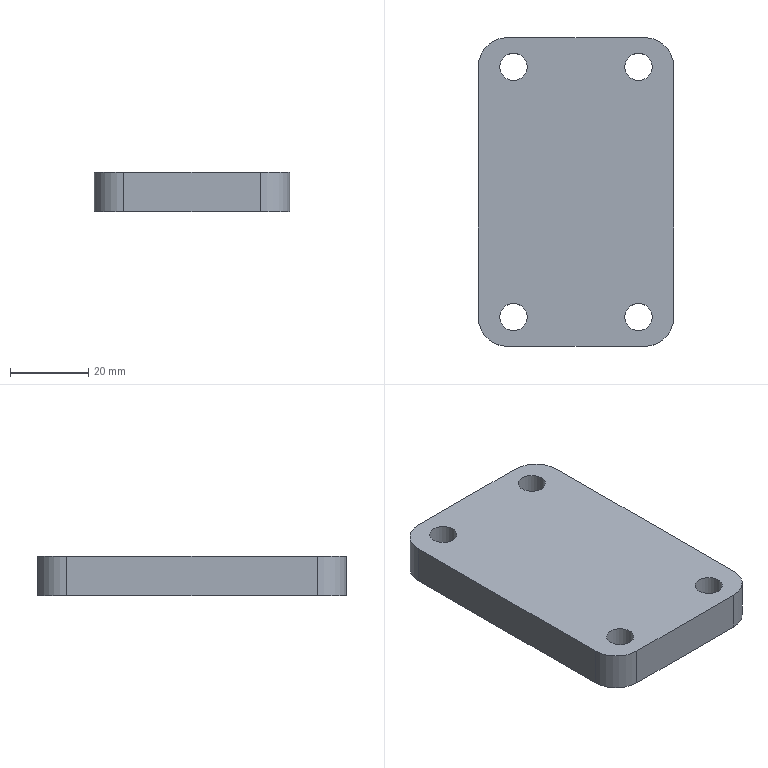Part | NX | features solid 2 | 1 solid | 14 faces | box 50 x 79 x 10 mm | volume 37478 mm3 | cylinder 8 | plane 6 | commonest cylinder face diameters 7 x4 15 x4
STEP:
#1=CARTESIAN_POINT('',(-542.5,-19.5,-137.));
#2=VERTEX_POINT('',#1);
#3=CARTESIAN_POINT('',(-577.5,-19.5,-137.));
#4=VERTEX_POINT('',#3);
#5=CARTESIAN_POINT('',(-535.,-19.5,-137.));
#6=DIRECTION('',(-1.,0.,0.));
#7=VECTOR('',#6,1000.);
#8=LINE('',#5,#7);
#9=EDGE_CURVE('',#2,#4,#8,.T.);
#10=ORIENTED_EDGE('',*,*,#9,.T.);
#11=CARTESIAN_POINT('',(-577.5,-19.5,-147.));
#12=VERTEX_POINT('',#11);
#13=CARTESIAN_POINT('',(-577.5,-19.5,-137.));
#14=DIRECTION('',(0.,0.,-1.));
#15=VECTOR('',#14,1000.);
#16=LINE('',#13,#15);
#17=EDGE_CURVE('',#4,#12,#16,.T.);
#18=ORIENTED_EDGE('',*,*,#17,.T.);
#19=CARTESIAN_POINT('',(-542.5,-19.5,-147.));
#20=VERTEX_POINT('',#19);
#21=CARTESIAN_POINT('',(-535.,-19.5,-147.));
#22=DIRECTION('',(-1.,0.,0.));
#23=VECTOR('',#22,1000.);
#24=LINE('',#21,#23);
#25=EDGE_CURVE('',#20,#12,#24,.T.);
#26=ORIENTED_EDGE('',*,*,#25,.F.);
#27=CARTESIAN_POINT('',(-542.5,-19.5,-137.));
#28=DIRECTION('',(0.,0.,-1.));
#29=VECTOR('',#28,1000.);
#30=LINE('',#27,#29);
#31=EDGE_CURVE('',#20,#2,#30,.F.);
#32=ORIENTED_EDGE('',*,*,#31,.T.);
#33=EDGE_LOOP('',(#10,#18,#26,#32));
#34=FACE_BOUND('',#33,.T.);
#35=CARTESIAN_POINT('',(-535.,-19.5,-137.));
#36=DIRECTION('',(0.,-1.,0.));
#37=DIRECTION('',(1.,0.,0.));
#38=AXIS2_PLACEMENT_3D('',#35,#36,#37);
#39=PLANE('',#38);
#40=ADVANCED_FACE('',(#34),#39,.T.);
#41=CARTESIAN_POINT('',(-585.,-12.,-137.));
#42=VERTEX_POINT('',#41);
#43=CARTESIAN_POINT('',(-585.,52.,-137.));
#44=VERTEX_POINT('',#43);
#45=CARTESIAN_POINT('',(-585.,-19.5,-137.));
#46=DIRECTION('',(0.,1.,0.));
#47=VECTOR('',#46,1000.);
#48=LINE('',#45,#47);
#49=EDGE_CURVE('',#42,#44,#48,.T.);
#50=ORIENTED_EDGE('',*,*,#49,.T.);
#51=CARTESIAN_POINT('',(-585.,52.,-147.));
#52=VERTEX_POINT('',#51);
#53=CARTESIAN_POINT('',(-585.,52.,-137.));
#54=DIRECTION('',(0.,0.,-1.));
#55=VECTOR('',#54,1000.);
#56=LINE('',#53,#55);
#57=EDGE_CURVE('',#44,#52,#56,.T.);
#58=ORIENTED_EDGE('',*,*,#57,.T.);
#59=CARTESIAN_POINT('',(-585.,-12.,-147.));
#60=VERTEX_POINT('',#59);
#61=CARTESIAN_POINT('',(-585.,-19.5,-147.));
#62=DIRECTION('',(0.,1.,0.));
#63=VECTOR('',#62,1000.);
#64=LINE('',#61,#63);
#65=EDGE_CURVE('',#60,#52,#64,.T.);
#66=ORIENTED_EDGE('',*,*,#65,.F.);
#67=CARTESIAN_POINT('',(-585.,-12.,-137.));
#68=DIRECTION('',(0.,0.,-1.));
#69=VECTOR('',#68,1000.);
#70=LINE('',#67,#69);
#71=EDGE_CURVE('',#60,#42,#70,.F.);
#72=ORIENTED_EDGE('',*,*,#71,.T.);
#73=EDGE_LOOP('',(#50,#58,#66,#72));
#74=FACE_BOUND('',#73,.T.);
#75=CARTESIAN_POINT('',(-585.,-19.5,-137.));
#76=DIRECTION('',(-1.,0.,0.));
#77=DIRECTION('',(0.,-1.,0.));
#78=AXIS2_PLACEMENT_3D('',#75,#76,#77);
#79=PLANE('',#78);
#80=ADVANCED_FACE('',(#74),#79,.T.);
#81=CARTESIAN_POINT('',(-577.5,59.5,-147.));
#82=VERTEX_POINT('',#81);
#83=CARTESIAN_POINT('',(-542.5,59.5,-147.));
#84=VERTEX_POINT('',#83);
#85=CARTESIAN_POINT('',(-585.,59.5,-147.));
#86=DIRECTION('',(1.,0.,0.));
#87=VECTOR('',#86,1000.);
#88=LINE('',#85,#87);
#89=EDGE_CURVE('',#82,#84,#88,.T.);
#90=ORIENTED_EDGE('',*,*,#89,.F.);
#91=CARTESIAN_POINT('',(-577.5,59.5,-137.));
#92=VERTEX_POINT('',#91);
#93=CARTESIAN_POINT('',(-577.5,59.5,-137.));
#94=DIRECTION('',(0.,0.,-1.));
#95=VECTOR('',#94,1000.);
#96=LINE('',#93,#95);
#97=EDGE_CURVE('',#82,#92,#96,.F.);
#98=ORIENTED_EDGE('',*,*,#97,.T.);
#99=CARTESIAN_POINT('',(-542.5,59.5,-137.));
#100=VERTEX_POINT('',#99);
#101=CARTESIAN_POINT('',(-585.,59.5,-137.));
#102=DIRECTION('',(1.,0.,0.));
#103=VECTOR('',#102,1000.);
#104=LINE('',#101,#103);
#105=EDGE_CURVE('',#92,#100,#104,.T.);
#106=ORIENTED_EDGE('',*,*,#105,.T.);
#107=CARTESIAN_POINT('',(-542.5,59.5,-137.));
#108=DIRECTION('',(0.,0.,-1.));
#109=VECTOR('',#108,1000.);
#110=LINE('',#107,#109);
#111=EDGE_CURVE('',#100,#84,#110,.T.);
#112=ORIENTED_EDGE('',*,*,#111,.T.);
#113=EDGE_LOOP('',(#90,#98,#106,#112));
#114=FACE_BOUND('',#113,.T.);
#115=CARTESIAN_POINT('',(-585.,59.5,-137.));
#116=DIRECTION('',(0.,1.,0.));
#117=DIRECTION('',(-1.,0.,0.));
#118=AXIS2_PLACEMENT_3D('',#115,#116,#117);
#119=PLANE('',#118);
#120=ADVANCED_FACE('',(#114),#119,.T.);
#121=CARTESIAN_POINT('',(-535.,52.,-147.));
#122=VERTEX_POINT('',#121);
#123=CARTESIAN_POINT('',(-535.,-12.,-147.));
#124=VERTEX_POINT('',#123);
#125=CARTESIAN_POINT('',(-535.,59.5,-147.));
#126=DIRECTION('',(0.,-1.,0.));
#127=VECTOR('',#126,1000.);
#128=LINE('',#125,#127);
#129=EDGE_CURVE('',#122,#124,#128,.T.);
#130=ORIENTED_EDGE('',*,*,#129,.F.);
#131=CARTESIAN_POINT('',(-535.,52.,-137.));
#132=VERTEX_POINT('',#131);
#133=CARTESIAN_POINT('',(-535.,52.,-137.));
#134=DIRECTION('',(0.,0.,-1.));
#135=VECTOR('',#134,1000.);
#136=LINE('',#133,#135);
#137=EDGE_CURVE('',#122,#132,#136,.F.);
#138=ORIENTED_EDGE('',*,*,#137,.T.);
#139=CARTESIAN_POINT('',(-535.,-12.,-137.));
#140=VERTEX_POINT('',#139);
#141=CARTESIAN_POINT('',(-535.,59.5,-137.));
#142=DIRECTION('',(0.,-1.,0.));
#143=VECTOR('',#142,1000.);
#144=LINE('',#141,#143);
#145=EDGE_CURVE('',#132,#140,#144,.T.);
#146=ORIENTED_EDGE('',*,*,#145,.T.);
#147=CARTESIAN_POINT('',(-535.,-12.,-137.));
#148=DIRECTION('',(0.,0.,-1.));
#149=VECTOR('',#148,1000.);
#150=LINE('',#147,#149);
#151=EDGE_CURVE('',#140,#124,#150,.T.);
#152=ORIENTED_EDGE('',*,*,#151,.T.);
#153=EDGE_LOOP('',(#130,#138,#146,#152));
#154=FACE_BOUND('',#153,.T.);
#155=CARTESIAN_POINT('',(-535.,59.5,-137.));
#156=DIRECTION('',(1.,0.,0.));
#157=DIRECTION('',(0.,1.,0.));
#158=AXIS2_PLACEMENT_3D('',#155,#156,#157);
#159=PLANE('',#158);
#160=ADVANCED_FACE('',(#154),#159,.T.);
#161=CARTESIAN_POINT('',(-544.,55.5,-137.));
#162=VERTEX_POINT('',#161);
#163=CARTESIAN_POINT('',(-544.,52.,-137.));
#164=DIRECTION('',(0.,0.,-1.));
#165=DIRECTION('',(0.,1.,0.));
#166=AXIS2_PLACEMENT_3D('',#163,#164,#165);
#167=CIRCLE('',#166,3.5);
#168=EDGE_CURVE('',#162,#162,#167,.T.);
#169=ORIENTED_EDGE('',*,*,#168,.T.);
#170=EDGE_LOOP('',(#169));
#171=FACE_BOUND('',#170,.T.);
#172=CARTESIAN_POINT('',(-576.,55.5,-137.));
#173=VERTEX_POINT('',#172);
#174=CARTESIAN_POINT('',(-576.,52.,-137.));
#175=DIRECTION('',(0.,0.,1.));
#176=DIRECTION('',(0.,1.,0.));
#177=AXIS2_PLACEMENT_3D('',#174,#175,#176);
#178=CIRCLE('',#177,3.5);
#179=EDGE_CURVE('',#173,#173,#178,.T.);
#180=ORIENTED_EDGE('',*,*,#179,.F.);
#181=EDGE_LOOP('',(#180));
#182=FACE_BOUND('',#181,.T.);
#183=CARTESIAN_POINT('',(-544.,-15.5,-137.));
#184=VERTEX_POINT('',#183);
#185=CARTESIAN_POINT('',(-544.,-12.,-137.));
#186=DIRECTION('',(0.,0.,1.));
#187=DIRECTION('',(0.,-1.,0.));
#188=AXIS2_PLACEMENT_3D('',#185,#186,#187);
#189=CIRCLE('',#188,3.5);
#190=EDGE_CURVE('',#184,#184,#189,.T.);
#191=ORIENTED_EDGE('',*,*,#190,.F.);
#192=EDGE_LOOP('',(#191));
#193=FACE_BOUND('',#192,.T.);
#194=CARTESIAN_POINT('',(-576.,-15.5,-137.));
#195=VERTEX_POINT('',#194);
#196=CARTESIAN_POINT('',(-576.,-12.,-137.));
#197=DIRECTION('',(0.,0.,-1.));
#198=DIRECTION('',(0.,-1.,0.));
#199=AXIS2_PLACEMENT_3D('',#196,#197,#198);
#200=CIRCLE('',#199,3.5);
#201=EDGE_CURVE('',#195,#195,#200,.T.);
#202=ORIENTED_EDGE('',*,*,#201,.T.);
#203=EDGE_LOOP('',(#202));
#204=FACE_BOUND('',#203,.T.);
#205=ORIENTED_EDGE('',*,*,#105,.F.);
#206=CARTESIAN_POINT('',(-577.5,52.,-137.));
#207=DIRECTION('',(0.,0.,1.));
#208=DIRECTION('',(0.,1.,0.));
#209=AXIS2_PLACEMENT_3D('',#206,#207,#208);
#210=CIRCLE('',#209,7.5);
#211=EDGE_CURVE('',#92,#44,#210,.T.);
#212=ORIENTED_EDGE('',*,*,#211,.T.);
#213=ORIENTED_EDGE('',*,*,#49,.F.);
#214=CARTESIAN_POINT('',(-577.5,-12.,-137.));
#215=DIRECTION('',(0.,0.,1.));
#216=DIRECTION('',(0.,1.,0.));
#217=AXIS2_PLACEMENT_3D('',#214,#215,#216);
#218=CIRCLE('',#217,7.5);
#219=EDGE_CURVE('',#42,#4,#218,.T.);
#220=ORIENTED_EDGE('',*,*,#219,.T.);
#221=ORIENTED_EDGE('',*,*,#9,.F.);
#222=CARTESIAN_POINT('',(-542.5,-12.,-137.));
#223=DIRECTION('',(0.,0.,1.));
#224=DIRECTION('',(0.,1.,0.));
#225=AXIS2_PLACEMENT_3D('',#222,#223,#224);
#226=CIRCLE('',#225,7.5);
#227=EDGE_CURVE('',#2,#140,#226,.T.);
#228=ORIENTED_EDGE('',*,*,#227,.T.);
#229=ORIENTED_EDGE('',*,*,#145,.F.);
#230=CARTESIAN_POINT('',(-542.5,52.,-137.));
#231=DIRECTION('',(0.,0.,1.));
#232=DIRECTION('',(0.,1.,0.));
#233=AXIS2_PLACEMENT_3D('',#230,#231,#232);
#234=CIRCLE('',#233,7.5);
#235=EDGE_CURVE('',#132,#100,#234,.T.);
#236=ORIENTED_EDGE('',*,*,#235,.T.);
#237=EDGE_LOOP('',(#205,#212,#213,#220,#221,#228,#229,#236));
#238=FACE_BOUND('',#237,.T.);
#239=CARTESIAN_POINT('',(-535.,-19.5,-137.));
#240=DIRECTION('',(0.,0.,1.));
#241=DIRECTION('',(0.,1.,0.));
#242=AXIS2_PLACEMENT_3D('',#239,#240,#241);
#243=PLANE('',#242);
#244=ADVANCED_FACE('',(#171,#182,#193,#204,#238),#243,.T.);
#245=CARTESIAN_POINT('',(-544.,55.5,-147.));
#246=VERTEX_POINT('',#245);
#247=CARTESIAN_POINT('',(-544.,52.,-147.));
#248=DIRECTION('',(0.,0.,-1.));
#249=DIRECTION('',(0.,1.,0.));
#250=AXIS2_PLACEMENT_3D('',#247,#248,#249);
#251=CIRCLE('',#250,3.5);
#252=EDGE_CURVE('',#246,#246,#251,.T.);
#253=ORIENTED_EDGE('',*,*,#252,.F.);
#254=EDGE_LOOP('',(#253));
#255=FACE_BOUND('',#254,.T.);
#256=CARTESIAN_POINT('',(-576.,55.5,-147.));
#257=VERTEX_POINT('',#256);
#258=CARTESIAN_POINT('',(-576.,52.,-147.));
#259=DIRECTION('',(0.,0.,1.));
#260=DIRECTION('',(0.,1.,0.));
#261=AXIS2_PLACEMENT_3D('',#258,#259,#260);
#262=CIRCLE('',#261,3.5);
#263=EDGE_CURVE('',#257,#257,#262,.T.);
#264=ORIENTED_EDGE('',*,*,#263,.T.);
#265=EDGE_LOOP('',(#264));
#266=FACE_BOUND('',#265,.T.);
#267=CARTESIAN_POINT('',(-544.,-15.5,-147.));
#268=VERTEX_POINT('',#267);
#269=CARTESIAN_POINT('',(-544.,-12.,-147.));
#270=DIRECTION('',(0.,0.,1.));
#271=DIRECTION('',(0.,-1.,0.));
#272=AXIS2_PLACEMENT_3D('',#269,#270,#271);
#273=CIRCLE('',#272,3.5);
#274=EDGE_CURVE('',#268,#268,#273,.T.);
#275=ORIENTED_EDGE('',*,*,#274,.T.);
#276=EDGE_LOOP('',(#275));
#277=FACE_BOUND('',#276,.T.);
#278=CARTESIAN_POINT('',(-576.,-15.5,-147.));
#279=VERTEX_POINT('',#278);
#280=CARTESIAN_POINT('',(-576.,-12.,-147.));
#281=DIRECTION('',(0.,0.,-1.));
#282=DIRECTION('',(0.,-1.,0.));
#283=AXIS2_PLACEMENT_3D('',#280,#281,#282);
#284=CIRCLE('',#283,3.5);
#285=EDGE_CURVE('',#279,#279,#284,.T.);
#286=ORIENTED_EDGE('',*,*,#285,.F.);
#287=EDGE_LOOP('',(#286));
#288=FACE_BOUND('',#287,.T.);
#289=ORIENTED_EDGE('',*,*,#65,.T.);
#290=CARTESIAN_POINT('',(-577.5,52.,-147.));
#291=DIRECTION('',(0.,0.,1.));
#292=DIRECTION('',(0.,1.,0.));
#293=AXIS2_PLACEMENT_3D('',#290,#291,#292);
#294=CIRCLE('',#293,7.5);
#295=EDGE_CURVE('',#52,#82,#294,.F.);
#296=ORIENTED_EDGE('',*,*,#295,.T.);
#297=ORIENTED_EDGE('',*,*,#89,.T.);
#298=CARTESIAN_POINT('',(-542.5,52.,-147.));
#299=DIRECTION('',(0.,0.,1.));
#300=DIRECTION('',(0.,1.,0.));
#301=AXIS2_PLACEMENT_3D('',#298,#299,#300);
#302=CIRCLE('',#301,7.5);
#303=EDGE_CURVE('',#84,#122,#302,.F.);
#304=ORIENTED_EDGE('',*,*,#303,.T.);
#305=ORIENTED_EDGE('',*,*,#129,.T.);
#306=CARTESIAN_POINT('',(-542.5,-12.,-147.));
#307=DIRECTION('',(0.,0.,1.));
#308=DIRECTION('',(0.,1.,0.));
#309=AXIS2_PLACEMENT_3D('',#306,#307,#308);
#310=CIRCLE('',#309,7.5);
#311=EDGE_CURVE('',#124,#20,#310,.F.);
#312=ORIENTED_EDGE('',*,*,#311,.T.);
#313=ORIENTED_EDGE('',*,*,#25,.T.);
#314=CARTESIAN_POINT('',(-577.5,-12.,-147.));
#315=DIRECTION('',(0.,0.,1.));
#316=DIRECTION('',(0.,1.,0.));
#317=AXIS2_PLACEMENT_3D('',#314,#315,#316);
#318=CIRCLE('',#317,7.5);
#319=EDGE_CURVE('',#12,#60,#318,.F.);
#320=ORIENTED_EDGE('',*,*,#319,.T.);
#321=EDGE_LOOP('',(#289,#296,#297,#304,#305,#312,#313,#320));
#322=FACE_BOUND('',#321,.T.);
#323=CARTESIAN_POINT('',(-535.,-19.5,-147.));
#324=DIRECTION('',(0.,0.,1.));
#325=DIRECTION('',(0.,1.,0.));
#326=AXIS2_PLACEMENT_3D('',#323,#324,#325);
#327=PLANE('',#326);
#328=ADVANCED_FACE('',(#255,#266,#277,#288,#322),#327,.F.);
#329=ORIENTED_EDGE('',*,*,#211,.F.);
#330=ORIENTED_EDGE('',*,*,#97,.F.);
#331=ORIENTED_EDGE('',*,*,#295,.F.);
#332=ORIENTED_EDGE('',*,*,#57,.F.);
#333=EDGE_LOOP('',(#329,#330,#331,#332));
#334=FACE_BOUND('',#333,.T.);
#335=CARTESIAN_POINT('',(-577.5,52.,-137.));
#336=DIRECTION('',(0.,0.,-1.));
#337=DIRECTION('',(0.,-1.,0.));
#338=AXIS2_PLACEMENT_3D('',#335,#336,#337);
#339=CYLINDRICAL_SURFACE('',#338,7.5);
#340=ADVANCED_FACE('',(#334),#339,.T.);
#341=ORIENTED_EDGE('',*,*,#235,.F.);
#342=ORIENTED_EDGE('',*,*,#137,.F.);
#343=ORIENTED_EDGE('',*,*,#303,.F.);
#344=ORIENTED_EDGE('',*,*,#111,.F.);
#345=EDGE_LOOP('',(#341,#342,#343,#344));
#346=FACE_BOUND('',#345,.T.);
#347=CARTESIAN_POINT('',(-542.5,52.,-137.));
#348=DIRECTION('',(0.,0.,-1.));
#349=DIRECTION('',(0.,-1.,0.));
#350=AXIS2_PLACEMENT_3D('',#347,#348,#349);
#351=CYLINDRICAL_SURFACE('',#350,7.5);
#352=ADVANCED_FACE('',(#346),#351,.T.);
#353=ORIENTED_EDGE('',*,*,#219,.F.);
#354=ORIENTED_EDGE('',*,*,#71,.F.);
#355=ORIENTED_EDGE('',*,*,#319,.F.);
#356=ORIENTED_EDGE('',*,*,#17,.F.);
#357=EDGE_LOOP('',(#353,#354,#355,#356));
#358=FACE_BOUND('',#357,.T.);
#359=CARTESIAN_POINT('',(-577.5,-12.,-137.));
#360=DIRECTION('',(0.,0.,-1.));
#361=DIRECTION('',(0.,-1.,0.));
#362=AXIS2_PLACEMENT_3D('',#359,#360,#361);
#363=CYLINDRICAL_SURFACE('',#362,7.5);
#364=ADVANCED_FACE('',(#358),#363,.T.);
#365=ORIENTED_EDGE('',*,*,#227,.F.);
#366=ORIENTED_EDGE('',*,*,#31,.F.);
#367=ORIENTED_EDGE('',*,*,#311,.F.);
#368=ORIENTED_EDGE('',*,*,#151,.F.);
#369=EDGE_LOOP('',(#365,#366,#367,#368));
#370=FACE_BOUND('',#369,.T.);
#371=CARTESIAN_POINT('',(-542.5,-12.,-137.));
#372=DIRECTION('',(0.,0.,-1.));
#373=DIRECTION('',(0.,-1.,0.));
#374=AXIS2_PLACEMENT_3D('',#371,#372,#373);
#375=CYLINDRICAL_SURFACE('',#374,7.5);
#376=ADVANCED_FACE('',(#370),#375,.T.);
#377=ORIENTED_EDGE('',*,*,#285,.T.);
#378=EDGE_LOOP('',(#377));
#379=FACE_BOUND('',#378,.T.);
#380=ORIENTED_EDGE('',*,*,#201,.F.);
#381=EDGE_LOOP('',(#380));
#382=FACE_BOUND('',#381,.T.);
#383=CARTESIAN_POINT('',(-576.,-12.,-137.));
#384=DIRECTION('',(0.,0.,-1.));
#385=DIRECTION('',(0.,-1.,0.));
#386=AXIS2_PLACEMENT_3D('',#383,#384,#385);
#387=CYLINDRICAL_SURFACE('',#386,3.5);
#388=ADVANCED_FACE('',(#379,#382),#387,.F.);
#389=ORIENTED_EDGE('',*,*,#274,.F.);
#390=EDGE_LOOP('',(#389));
#391=FACE_BOUND('',#390,.T.);
#392=ORIENTED_EDGE('',*,*,#190,.T.);
#393=EDGE_LOOP('',(#392));
#394=FACE_BOUND('',#393,.T.);
#395=CARTESIAN_POINT('',(-544.,-12.,-137.));
#396=DIRECTION('',(0.,0.,-1.));
#397=DIRECTION('',(0.,-1.,0.));
#398=AXIS2_PLACEMENT_3D('',#395,#396,#397);
#399=CYLINDRICAL_SURFACE('',#398,3.5);
#400=ADVANCED_FACE('',(#391,#394),#399,.F.);
#401=ORIENTED_EDGE('',*,*,#263,.F.);
#402=EDGE_LOOP('',(#401));
#403=FACE_BOUND('',#402,.T.);
#404=ORIENTED_EDGE('',*,*,#179,.T.);
#405=EDGE_LOOP('',(#404));
#406=FACE_BOUND('',#405,.T.);
#407=CARTESIAN_POINT('',(-576.,52.,-137.));
#408=DIRECTION('',(0.,0.,-1.));
#409=DIRECTION('',(0.,1.,0.));
#410=AXIS2_PLACEMENT_3D('',#407,#408,#409);
#411=CYLINDRICAL_SURFACE('',#410,3.5);
#412=ADVANCED_FACE('',(#403,#406),#411,.F.);
#413=ORIENTED_EDGE('',*,*,#252,.T.);
#414=EDGE_LOOP('',(#413));
#415=FACE_BOUND('',#414,.T.);
#416=ORIENTED_EDGE('',*,*,#168,.F.);
#417=EDGE_LOOP('',(#416));
#418=FACE_BOUND('',#417,.T.);
#419=CARTESIAN_POINT('',(-544.,52.,-137.));
#420=DIRECTION('',(0.,0.,-1.));
#421=DIRECTION('',(0.,1.,0.));
#422=AXIS2_PLACEMENT_3D('',#419,#420,#421);
#423=CYLINDRICAL_SURFACE('',#422,3.5);
#424=ADVANCED_FACE('',(#415,#418),#423,.F.);
#425=CLOSED_SHELL('',(#40,#80,#120,#160,#244,#328,#340,#352,#364,#376,#388,#400,#412,#424));
#426=MANIFOLD_SOLID_BREP('',#425);
#427=(LENGTH_UNIT()NAMED_UNIT(*)SI_UNIT(.MILLI.,.METRE.));
#428=UNCERTAINTY_MEASURE_WITH_UNIT(LENGTH_MEASURE(0.00001),#427,'','');
#429=(NAMED_UNIT(*)PLANE_ANGLE_UNIT()SI_UNIT($,.RADIAN.));
#430=(NAMED_UNIT(*)SI_UNIT($,.STERADIAN.)SOLID_ANGLE_UNIT());
#431=(GEOMETRIC_REPRESENTATION_CONTEXT(3)GLOBAL_UNCERTAINTY_ASSIGNED_CONTEXT((#428))GLOBAL_UNIT_ASSIGNED_CONTEXT((#427,#429,#430))REPRESENTATION_CONTEXT('',''));
#432=ADVANCED_BREP_SHAPE_REPRESENTATION('',(#426),#431);